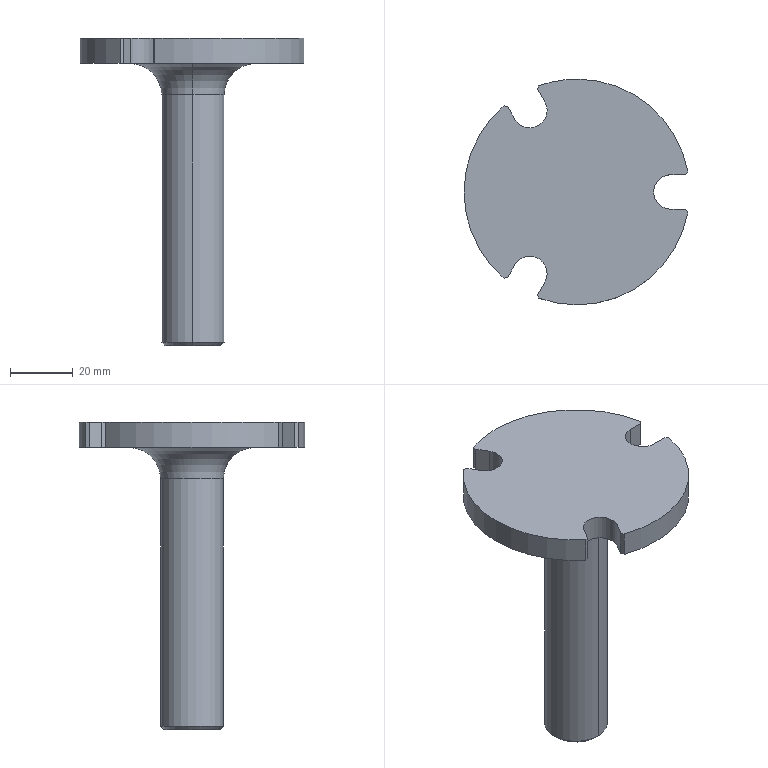CAM job | NX | 3-axis milling | part box 71.434 x 72 x 98 mm | stock box 72 x 72 x 98 mm
Tools:
number,name,description,diameter,corner_radius,flute_length,length,flutes
6,D6C,Milling Tool-5 Parameters,6.0,0.0,50.0,75.0,2
8,D6JING,Milling Tool-5 Parameters,6.0,0.0,50.0,75.0,2
7,D6A45,Milling Tool-5 Parameters,6.0,0.0,50.0,75.0,2
Operations:
program,operation,operation_type,tool,method,geometry_group,spindle_rpm,surface_speed,feed_per_tooth,feed_cut,feed_plunge,cut_length_mm,path_length_mm,cut_time_min,machine_time_min
1,ZLEVEL_PROFILE_COPY_1,ZLevelMilling,D6C,METHOD,A,5000.0,94.0,0.18,1800.0,100.0,18237.542,25512.884,10.132,10.86
1,ZLEVEL_PROFILE_COPY,ZLevelMilling,D6JING,METHOD,A,7500.0,141.0,0.0667,1000.0,100.0,109.888,490.947,0.1099,0.148
1,PLANAR_MILL_COPY,PlanarMilling,D6A45,METHOD,A,7500.0,141.0,0.0833,1250.0,100.0,102.438,398.901,0.082,0.1116